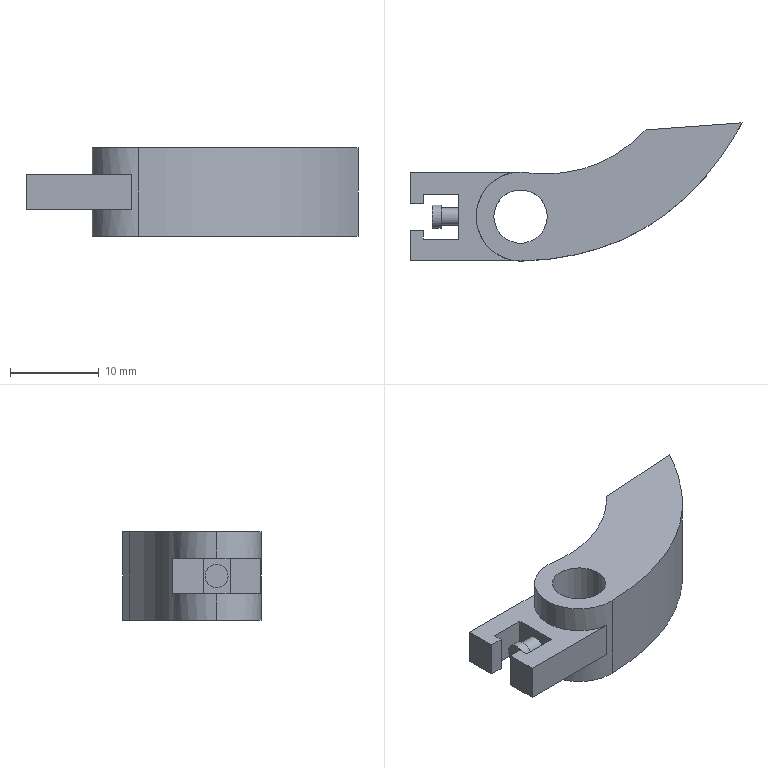Part | SolidWorks | features ICE 6, Extrusion 1 | 1 solid | 28 faces | box 37.304 x 15.525 x 10 mm | volume 2448 mm3 | plane 18 | cylinder 8 | spline 2 | commonest cylinder face diameters 2 x2 2.6 x2 6 x2 10 x2
STEP:
#1=CARTESIAN_POINT('',(-8.923,-1.3,5.));
#2=VERTEX_POINT('',#1);
#3=CARTESIAN_POINT('',(-8.923,1.3,5.));
#4=VERTEX_POINT('',#3);
#5=CARTESIAN_POINT('',(-8.923,0.,5.));
#6=DIRECTION('',(-1.,0.,0.));
#7=DIRECTION('',(0.,-1.,0.));
#8=AXIS2_PLACEMENT_3D('',#5,#6,#7);
#9=CIRCLE('',#8,1.3);
#10=EDGE_CURVE('',#2,#4,#9,.T.);
#11=ORIENTED_EDGE('',*,*,#10,.T.);
#12=CARTESIAN_POINT('',(-9.923,1.3,5.));
#13=VERTEX_POINT('',#12);
#14=CARTESIAN_POINT('',(-8.923,1.3,5.));
#15=DIRECTION('',(-1.,0.,0.));
#16=VECTOR('',#15,1000.);
#17=LINE('',#14,#16);
#18=EDGE_CURVE('',#4,#13,#17,.T.);
#19=ORIENTED_EDGE('',*,*,#18,.T.);
#20=CARTESIAN_POINT('',(-9.923,-1.3,5.));
#21=VERTEX_POINT('',#20);
#22=CARTESIAN_POINT('',(-9.923,0.,5.));
#23=DIRECTION('',(-1.,0.,0.));
#24=DIRECTION('',(0.,-1.,0.));
#25=AXIS2_PLACEMENT_3D('',#22,#23,#24);
#26=CIRCLE('',#25,1.3);
#27=EDGE_CURVE('',#21,#13,#26,.T.);
#28=ORIENTED_EDGE('',*,*,#27,.F.);
#29=CARTESIAN_POINT('',(-8.923,-1.3,5.));
#30=DIRECTION('',(-1.,0.,0.));
#31=VECTOR('',#30,1000.);
#32=LINE('',#29,#31);
#33=EDGE_CURVE('',#2,#21,#32,.T.);
#34=ORIENTED_EDGE('',*,*,#33,.F.);
#35=EDGE_LOOP('',(#11,#19,#28,#34));
#36=FACE_OUTER_BOUND('',#35,.T.);
#37=CARTESIAN_POINT('',(-8.923,0.,5.));
#38=DIRECTION('',(-1.,0.,0.));
#39=DIRECTION('',(0.,-1.,0.));
#40=AXIS2_PLACEMENT_3D('',#37,#38,#39);
#41=CYLINDRICAL_SURFACE('',#40,1.3);
#42=ADVANCED_FACE('',(#36),#41,.T.);
#43=CARTESIAN_POINT('',(-3.,0.,10.));
#44=VERTEX_POINT('',#43);
#45=CARTESIAN_POINT('',(3.,0.,10.));
#46=VERTEX_POINT('',#45);
#47=CARTESIAN_POINT('',(0.,0.,10.));
#48=DIRECTION('',(0.,0.,1.));
#49=DIRECTION('',(1.,0.,0.));
#50=AXIS2_PLACEMENT_3D('',#47,#48,#49);
#51=CIRCLE('',#50,3.);
#52=EDGE_CURVE('',#44,#46,#51,.T.);
#53=ORIENTED_EDGE('',*,*,#52,.T.);
#54=CARTESIAN_POINT('',(3.,0.,0.));
#55=VERTEX_POINT('',#54);
#56=CARTESIAN_POINT('',(3.,0.,10.));
#57=DIRECTION('',(0.,0.,-1.));
#58=VECTOR('',#57,1000.);
#59=LINE('',#56,#58);
#60=EDGE_CURVE('',#46,#55,#59,.T.);
#61=ORIENTED_EDGE('',*,*,#60,.T.);
#62=CARTESIAN_POINT('',(-3.,0.,0.));
#63=VERTEX_POINT('',#62);
#64=CARTESIAN_POINT('',(0.,0.,0.));
#65=DIRECTION('',(0.,0.,1.));
#66=DIRECTION('',(1.,0.,0.));
#67=AXIS2_PLACEMENT_3D('',#64,#65,#66);
#68=CIRCLE('',#67,3.);
#69=EDGE_CURVE('',#63,#55,#68,.T.);
#70=ORIENTED_EDGE('',*,*,#69,.F.);
#71=CARTESIAN_POINT('',(-3.,0.,10.));
#72=DIRECTION('',(0.,0.,-1.));
#73=VECTOR('',#72,1000.);
#74=LINE('',#71,#73);
#75=EDGE_CURVE('',#44,#63,#74,.T.);
#76=ORIENTED_EDGE('',*,*,#75,.F.);
#77=EDGE_LOOP('',(#53,#61,#70,#76));
#78=FACE_OUTER_BOUND('',#77,.T.);
#79=CARTESIAN_POINT('',(0.,0.,10.));
#80=DIRECTION('',(0.,0.,-1.));
#81=DIRECTION('',(-1.,0.,0.));
#82=AXIS2_PLACEMENT_3D('',#79,#80,#81);
#83=CYLINDRICAL_SURFACE('',#82,3.);
#84=ADVANCED_FACE('',(#78),#83,.F.);
#85=CARTESIAN_POINT('',(-5.,0.,10.));
#86=VERTEX_POINT('',#85);
#87=CARTESIAN_POINT('',(0.,-5.,10.));
#88=VERTEX_POINT('',#87);
#89=CARTESIAN_POINT('',(0.,0.,10.));
#90=DIRECTION('',(0.,0.,1.));
#91=DIRECTION('',(1.,0.,0.));
#92=AXIS2_PLACEMENT_3D('',#89,#90,#91);
#93=CIRCLE('',#92,5.);
#94=EDGE_CURVE('',#86,#88,#93,.T.);
#95=ORIENTED_EDGE('',*,*,#94,.F.);
#96=CARTESIAN_POINT('',(-5.,0.,7.));
#97=VERTEX_POINT('',#96);
#98=CARTESIAN_POINT('',(-5.,0.,10.));
#99=DIRECTION('',(0.,0.,-1.));
#100=VECTOR('',#99,1000.);
#101=LINE('',#98,#100);
#102=EDGE_CURVE('',#86,#97,#101,.T.);
#103=ORIENTED_EDGE('',*,*,#102,.T.);
#104=CARTESIAN_POINT('',(-0.589,-4.965,7.));
#105=VERTEX_POINT('',#104);
#106=CARTESIAN_POINT('',(0.,0.,7.));
#107=DIRECTION('',(0.,0.,1.));
#108=DIRECTION('',(1.,0.,0.));
#109=AXIS2_PLACEMENT_3D('',#106,#107,#108);
#110=CIRCLE('',#109,5.);
#111=EDGE_CURVE('',#97,#105,#110,.T.);
#112=ORIENTED_EDGE('',*,*,#111,.T.);
#113=CARTESIAN_POINT('',(-0.589,-4.965,3.));
#114=VERTEX_POINT('',#113);
#115=CARTESIAN_POINT('',(-0.589,-4.965,10.));
#116=DIRECTION('',(0.,0.,-1.));
#117=VECTOR('',#116,1000.);
#118=LINE('',#115,#117);
#119=EDGE_CURVE('',#105,#114,#118,.T.);
#120=ORIENTED_EDGE('',*,*,#119,.T.);
#121=CARTESIAN_POINT('',(-5.,0.,3.));
#122=VERTEX_POINT('',#121);
#123=CARTESIAN_POINT('',(0.,0.,3.));
#124=DIRECTION('',(0.,0.,1.));
#125=DIRECTION('',(1.,0.,0.));
#126=AXIS2_PLACEMENT_3D('',#123,#124,#125);
#127=CIRCLE('',#126,5.);
#128=EDGE_CURVE('',#122,#114,#127,.T.);
#129=ORIENTED_EDGE('',*,*,#128,.F.);
#130=CARTESIAN_POINT('',(-5.,0.,0.));
#131=VERTEX_POINT('',#130);
#132=CARTESIAN_POINT('',(-5.,0.,10.));
#133=DIRECTION('',(0.,0.,-1.));
#134=VECTOR('',#133,1000.);
#135=LINE('',#132,#134);
#136=EDGE_CURVE('',#122,#131,#135,.T.);
#137=ORIENTED_EDGE('',*,*,#136,.T.);
#138=CARTESIAN_POINT('',(0.,-5.,0.));
#139=VERTEX_POINT('',#138);
#140=CARTESIAN_POINT('',(0.,0.,0.));
#141=DIRECTION('',(0.,0.,1.));
#142=DIRECTION('',(1.,0.,0.));
#143=AXIS2_PLACEMENT_3D('',#140,#141,#142);
#144=CIRCLE('',#143,5.);
#145=EDGE_CURVE('',#131,#139,#144,.T.);
#146=ORIENTED_EDGE('',*,*,#145,.T.);
#147=CARTESIAN_POINT('',(0.2548,-4.994,0.));
#148=VERTEX_POINT('',#147);
#149=CARTESIAN_POINT('',(0.,-5.,0.));
#150=CARTESIAN_POINT('',(0.08497,-5.,0.));
#151=CARTESIAN_POINT('',(0.1699,-4.998,0.));
#152=CARTESIAN_POINT('',(0.2548,-4.994,0.));
#153=B_SPLINE_CURVE_WITH_KNOTS('',3,(#149,#150,#151,#152),.UNSPECIFIED.,.F.,.F.,(4,4),(0.,1.),.UNSPECIFIED.);
#154=EDGE_CURVE('',#139,#148,#153,.T.);
#155=ORIENTED_EDGE('',*,*,#154,.T.);
#156=CARTESIAN_POINT('',(0.2548,-4.994,10.));
#157=VERTEX_POINT('',#156);
#158=CARTESIAN_POINT('',(0.2548,-4.994,0.));
#159=DIRECTION('',(0.,0.,1.));
#160=VECTOR('',#159,1000.);
#161=LINE('',#158,#160);
#162=EDGE_CURVE('',#148,#157,#161,.T.);
#163=ORIENTED_EDGE('',*,*,#162,.T.);
#164=CARTESIAN_POINT('',(0.,-5.,10.));
#165=CARTESIAN_POINT('',(0.08493,-4.998,10.));
#166=CARTESIAN_POINT('',(0.1699,-4.996,10.));
#167=CARTESIAN_POINT('',(0.2548,-4.994,10.));
#168=B_SPLINE_CURVE_WITH_KNOTS('',3,(#164,#165,#166,#167),.UNSPECIFIED.,.F.,.F.,(4,4),(0.,1.),.UNSPECIFIED.);
#169=EDGE_CURVE('',#88,#157,#168,.T.);
#170=ORIENTED_EDGE('',*,*,#169,.F.);
#171=EDGE_LOOP('',(#95,#103,#112,#120,#129,#137,#146,#155,#163,#170));
#172=FACE_OUTER_BOUND('',#171,.T.);
#173=CARTESIAN_POINT('',(0.,0.,10.));
#174=DIRECTION('',(0.,0.,-1.));
#175=DIRECTION('',(-1.,0.,0.));
#176=AXIS2_PLACEMENT_3D('',#173,#174,#175);
#177=CYLINDRICAL_SURFACE('',#176,5.);
#178=ADVANCED_FACE('',(#172),#177,.T.);
#179=CARTESIAN_POINT('',(-8.923,-1.,5.));
#180=VERTEX_POINT('',#179);
#181=CARTESIAN_POINT('',(-8.923,1.,5.));
#182=VERTEX_POINT('',#181);
#183=CARTESIAN_POINT('',(-8.923,0.,5.));
#184=DIRECTION('',(-1.,0.,0.));
#185=DIRECTION('',(0.,-1.,0.));
#186=AXIS2_PLACEMENT_3D('',#183,#184,#185);
#187=CIRCLE('',#186,1.);
#188=EDGE_CURVE('',#180,#182,#187,.T.);
#189=ORIENTED_EDGE('',*,*,#188,.F.);
#190=CARTESIAN_POINT('',(-6.923,-1.,5.));
#191=VERTEX_POINT('',#190);
#192=CARTESIAN_POINT('',(-9.923,-1.,5.));
#193=DIRECTION('',(1.,0.,0.));
#194=VECTOR('',#193,1000.);
#195=LINE('',#192,#194);
#196=EDGE_CURVE('',#180,#191,#195,.T.);
#197=ORIENTED_EDGE('',*,*,#196,.T.);
#198=CARTESIAN_POINT('',(-6.923,1.,5.));
#199=VERTEX_POINT('',#198);
#200=CARTESIAN_POINT('',(-6.923,0.,5.));
#201=DIRECTION('',(-1.,0.,0.));
#202=DIRECTION('',(0.,1.,0.));
#203=AXIS2_PLACEMENT_3D('',#200,#201,#202);
#204=CIRCLE('',#203,1.);
#205=EDGE_CURVE('',#191,#199,#204,.T.);
#206=ORIENTED_EDGE('',*,*,#205,.T.);
#207=CARTESIAN_POINT('',(-9.923,1.,5.));
#208=DIRECTION('',(1.,0.,0.));
#209=VECTOR('',#208,1000.);
#210=LINE('',#207,#209);
#211=EDGE_CURVE('',#182,#199,#210,.T.);
#212=ORIENTED_EDGE('',*,*,#211,.F.);
#213=EDGE_LOOP('',(#189,#197,#206,#212));
#214=FACE_OUTER_BOUND('',#213,.T.);
#215=CARTESIAN_POINT('',(-9.923,0.,5.));
#216=DIRECTION('',(1.,0.,0.));
#217=DIRECTION('',(0.,1.,0.));
#218=AXIS2_PLACEMENT_3D('',#215,#216,#217);
#219=CYLINDRICAL_SURFACE('',#218,1.);
#220=ADVANCED_FACE('',(#214),#219,.T.);
#221=ORIENTED_EDGE('',*,*,#196,.F.);
#222=CARTESIAN_POINT('',(-8.923,0.,5.));
#223=DIRECTION('',(-1.,0.,0.));
#224=DIRECTION('',(0.,-1.,0.));
#225=AXIS2_PLACEMENT_3D('',#222,#223,#224);
#226=CIRCLE('',#225,1.);
#227=EDGE_CURVE('',#182,#180,#226,.T.);
#228=ORIENTED_EDGE('',*,*,#227,.F.);
#229=ORIENTED_EDGE('',*,*,#211,.T.);
#230=CARTESIAN_POINT('',(-6.923,0.,5.));
#231=DIRECTION('',(-1.,0.,0.));
#232=DIRECTION('',(0.,1.,0.));
#233=AXIS2_PLACEMENT_3D('',#230,#231,#232);
#234=CIRCLE('',#233,1.);
#235=EDGE_CURVE('',#199,#191,#234,.T.);
#236=ORIENTED_EDGE('',*,*,#235,.T.);
#237=EDGE_LOOP('',(#221,#228,#229,#236));
#238=FACE_OUTER_BOUND('',#237,.T.);
#239=CARTESIAN_POINT('',(-9.923,0.,5.));
#240=DIRECTION('',(1.,0.,0.));
#241=DIRECTION('',(0.,1.,0.));
#242=AXIS2_PLACEMENT_3D('',#239,#240,#241);
#243=CYLINDRICAL_SURFACE('',#242,1.);
#244=ADVANCED_FACE('',(#238),#243,.T.);
#245=CARTESIAN_POINT('',(-12.423,1.465,7.));
#246=VERTEX_POINT('',#245);
#247=CARTESIAN_POINT('',(-12.423,1.465,3.));
#248=VERTEX_POINT('',#247);
#249=CARTESIAN_POINT('',(-12.423,1.465,0.));
#250=DIRECTION('',(0.,0.,-1.));
#251=VECTOR('',#250,1000.);
#252=LINE('',#249,#251);
#253=EDGE_CURVE('',#246,#248,#252,.T.);
#254=ORIENTED_EDGE('',*,*,#253,.F.);
#255=CARTESIAN_POINT('',(-12.423,4.965,7.));
#256=VERTEX_POINT('',#255);
#257=CARTESIAN_POINT('',(-12.423,4.965,7.));
#258=DIRECTION('',(0.,1.,0.));
#259=VECTOR('',#258,1000.);
#260=LINE('',#257,#259);
#261=EDGE_CURVE('',#246,#256,#260,.T.);
#262=ORIENTED_EDGE('',*,*,#261,.T.);
#263=CARTESIAN_POINT('',(-12.423,4.965,3.));
#264=VERTEX_POINT('',#263);
#265=CARTESIAN_POINT('',(-12.423,4.965,3.));
#266=DIRECTION('',(0.,0.,-1.));
#267=VECTOR('',#266,1000.);
#268=LINE('',#265,#267);
#269=EDGE_CURVE('',#256,#264,#268,.T.);
#270=ORIENTED_EDGE('',*,*,#269,.T.);
#271=CARTESIAN_POINT('',(-12.423,4.965,3.));
#272=DIRECTION('',(0.,-1.,0.));
#273=VECTOR('',#272,1000.);
#274=LINE('',#271,#273);
#275=EDGE_CURVE('',#264,#248,#274,.T.);
#276=ORIENTED_EDGE('',*,*,#275,.T.);
#277=EDGE_LOOP('',(#254,#262,#270,#276));
#278=FACE_OUTER_BOUND('',#277,.T.);
#279=CARTESIAN_POINT('',(-12.423,0.,0.));
#280=DIRECTION('',(-1.,0.,0.));
#281=DIRECTION('',(0.,0.,1.));
#282=AXIS2_PLACEMENT_3D('',#279,#280,#281);
#283=PLANE('',#282);
#284=ADVANCED_FACE('',(#278),#283,.T.);
#285=CARTESIAN_POINT('',(-12.423,-4.965,7.));
#286=VERTEX_POINT('',#285);
#287=CARTESIAN_POINT('',(-20.423,-4.965,7.));
#288=DIRECTION('',(1.,0.,0.));
#289=VECTOR('',#288,1000.);
#290=LINE('',#287,#289);
#291=EDGE_CURVE('',#286,#105,#290,.T.);
#292=ORIENTED_EDGE('',*,*,#291,.F.);
#293=CARTESIAN_POINT('',(-12.423,-4.965,3.));
#294=VERTEX_POINT('',#293);
#295=CARTESIAN_POINT('',(-12.423,-4.965,3.));
#296=DIRECTION('',(0.,0.,1.));
#297=VECTOR('',#296,1000.);
#298=LINE('',#295,#297);
#299=EDGE_CURVE('',#294,#286,#298,.T.);
#300=ORIENTED_EDGE('',*,*,#299,.F.);
#301=CARTESIAN_POINT('',(-20.423,-4.965,3.));
#302=DIRECTION('',(1.,0.,0.));
#303=VECTOR('',#302,1000.);
#304=LINE('',#301,#303);
#305=EDGE_CURVE('',#294,#114,#304,.T.);
#306=ORIENTED_EDGE('',*,*,#305,.T.);
#307=ORIENTED_EDGE('',*,*,#119,.F.);
#308=EDGE_LOOP('',(#292,#300,#306,#307));
#309=FACE_OUTER_BOUND('',#308,.T.);
#310=CARTESIAN_POINT('',(-20.423,-4.965,3.));
#311=DIRECTION('',(0.,-1.,0.));
#312=DIRECTION('',(0.,0.,-1.));
#313=AXIS2_PLACEMENT_3D('',#310,#311,#312);
#314=PLANE('',#313);
#315=ADVANCED_FACE('',(#309),#314,.T.);
#316=CARTESIAN_POINT('',(-0.589,4.965,3.));
#317=VERTEX_POINT('',#316);
#318=CARTESIAN_POINT('',(-20.423,4.965,3.));
#319=DIRECTION('',(-1.,0.,0.));
#320=VECTOR('',#319,1000.);
#321=LINE('',#318,#320);
#322=EDGE_CURVE('',#317,#264,#321,.T.);
#323=ORIENTED_EDGE('',*,*,#322,.T.);
#324=ORIENTED_EDGE('',*,*,#269,.F.);
#325=CARTESIAN_POINT('',(-0.589,4.965,7.));
#326=VERTEX_POINT('',#325);
#327=CARTESIAN_POINT('',(-20.423,4.965,7.));
#328=DIRECTION('',(-1.,0.,0.));
#329=VECTOR('',#328,1000.);
#330=LINE('',#327,#329);
#331=EDGE_CURVE('',#326,#256,#330,.T.);
#332=ORIENTED_EDGE('',*,*,#331,.F.);
#333=CARTESIAN_POINT('',(-0.589,4.965,10.));
#334=DIRECTION('',(0.,0.,1.));
#335=VECTOR('',#334,1000.);
#336=LINE('',#333,#335);
#337=EDGE_CURVE('',#317,#326,#336,.T.);
#338=ORIENTED_EDGE('',*,*,#337,.F.);
#339=EDGE_LOOP('',(#323,#324,#332,#338));
#340=FACE_OUTER_BOUND('',#339,.T.);
#341=CARTESIAN_POINT('',(-20.423,4.965,3.));
#342=DIRECTION('',(0.,1.,0.));
#343=DIRECTION('',(0.,0.,1.));
#344=AXIS2_PLACEMENT_3D('',#341,#342,#343);
#345=PLANE('',#344);
#346=ADVANCED_FACE('',(#340),#345,.T.);
#347=CARTESIAN_POINT('',(-10.923,2.465,3.));
#348=VERTEX_POINT('',#347);
#349=CARTESIAN_POINT('',(-10.923,1.465,3.));
#350=VERTEX_POINT('',#349);
#351=CARTESIAN_POINT('',(-10.923,0.,3.));
#352=DIRECTION('',(0.,-1.,0.));
#353=VECTOR('',#352,1000.);
#354=LINE('',#351,#353);
#355=EDGE_CURVE('',#348,#350,#354,.T.);
#356=ORIENTED_EDGE('',*,*,#355,.T.);
#357=CARTESIAN_POINT('',(0.,1.465,3.));
#358=DIRECTION('',(-1.,0.,0.));
#359=VECTOR('',#358,1000.);
#360=LINE('',#357,#359);
#361=EDGE_CURVE('',#350,#248,#360,.T.);
#362=ORIENTED_EDGE('',*,*,#361,.T.);
#363=ORIENTED_EDGE('',*,*,#275,.F.);
#364=ORIENTED_EDGE('',*,*,#322,.F.);
#365=CARTESIAN_POINT('',(0.,0.,3.));
#366=DIRECTION('',(0.,0.,1.));
#367=DIRECTION('',(1.,0.,0.));
#368=AXIS2_PLACEMENT_3D('',#365,#366,#367);
#369=CIRCLE('',#368,5.);
#370=EDGE_CURVE('',#317,#122,#369,.T.);
#371=ORIENTED_EDGE('',*,*,#370,.T.);
#372=ORIENTED_EDGE('',*,*,#128,.T.);
#373=ORIENTED_EDGE('',*,*,#305,.F.);
#374=CARTESIAN_POINT('',(-12.423,-1.535,3.));
#375=VERTEX_POINT('',#374);
#376=CARTESIAN_POINT('',(-12.423,4.965,3.));
#377=DIRECTION('',(0.,-1.,0.));
#378=VECTOR('',#377,1000.);
#379=LINE('',#376,#378);
#380=EDGE_CURVE('',#375,#294,#379,.T.);
#381=ORIENTED_EDGE('',*,*,#380,.F.);
#382=CARTESIAN_POINT('',(-10.923,-1.535,3.));
#383=VERTEX_POINT('',#382);
#384=CARTESIAN_POINT('',(0.,-1.535,3.));
#385=DIRECTION('',(1.,0.,0.));
#386=VECTOR('',#385,1000.);
#387=LINE('',#384,#386);
#388=EDGE_CURVE('',#375,#383,#387,.T.);
#389=ORIENTED_EDGE('',*,*,#388,.T.);
#390=CARTESIAN_POINT('',(-10.923,-2.535,3.));
#391=VERTEX_POINT('',#390);
#392=CARTESIAN_POINT('',(-10.923,0.,3.));
#393=DIRECTION('',(0.,-1.,0.));
#394=VECTOR('',#393,1000.);
#395=LINE('',#392,#394);
#396=EDGE_CURVE('',#383,#391,#395,.T.);
#397=ORIENTED_EDGE('',*,*,#396,.T.);
#398=CARTESIAN_POINT('',(-6.923,-2.535,3.));
#399=VERTEX_POINT('',#398);
#400=CARTESIAN_POINT('',(0.,-2.535,3.));
#401=DIRECTION('',(1.,0.,0.));
#402=VECTOR('',#401,1000.);
#403=LINE('',#400,#402);
#404=EDGE_CURVE('',#391,#399,#403,.T.);
#405=ORIENTED_EDGE('',*,*,#404,.T.);
#406=CARTESIAN_POINT('',(-6.923,2.465,3.));
#407=VERTEX_POINT('',#406);
#408=CARTESIAN_POINT('',(-6.923,0.,3.));
#409=DIRECTION('',(0.,1.,0.));
#410=VECTOR('',#409,1000.);
#411=LINE('',#408,#410);
#412=EDGE_CURVE('',#399,#407,#411,.T.);
#413=ORIENTED_EDGE('',*,*,#412,.T.);
#414=CARTESIAN_POINT('',(0.,2.465,3.));
#415=DIRECTION('',(-1.,0.,0.));
#416=VECTOR('',#415,1000.);
#417=LINE('',#414,#416);
#418=EDGE_CURVE('',#407,#348,#417,.T.);
#419=ORIENTED_EDGE('',*,*,#418,.T.);
#420=EDGE_LOOP('',(#356,#362,#363,#364,#371,#372,#373,#381,#389,#397,#405,#413,#419));
#421=FACE_OUTER_BOUND('',#420,.T.);
#422=CARTESIAN_POINT('',(0.,0.,3.));
#423=DIRECTION('',(0.,0.,1.));
#424=DIRECTION('',(1.,0.,0.));
#425=AXIS2_PLACEMENT_3D('',#422,#423,#424);
#426=PLANE('',#425);
#427=ADVANCED_FACE('',(#421),#426,.F.);
#428=CARTESIAN_POINT('',(-10.923,1.465,7.));
#429=VERTEX_POINT('',#428);
#430=CARTESIAN_POINT('',(-12.423,1.465,7.));
#431=DIRECTION('',(-1.,0.,0.));
#432=VECTOR('',#431,1000.);
#433=LINE('',#430,#432);
#434=EDGE_CURVE('',#429,#246,#433,.T.);
#435=ORIENTED_EDGE('',*,*,#434,.F.);
#436=CARTESIAN_POINT('',(-10.923,2.465,7.));
#437=VERTEX_POINT('',#436);
#438=CARTESIAN_POINT('',(-10.923,1.465,7.));
#439=DIRECTION('',(0.,-1.,0.));
#440=VECTOR('',#439,1000.);
#441=LINE('',#438,#440);
#442=EDGE_CURVE('',#437,#429,#441,.T.);
#443=ORIENTED_EDGE('',*,*,#442,.F.);
#444=CARTESIAN_POINT('',(-6.923,2.465,7.));
#445=VERTEX_POINT('',#444);
#446=CARTESIAN_POINT('',(-10.923,2.465,7.));
#447=DIRECTION('',(-1.,0.,0.));
#448=VECTOR('',#447,1000.);
#449=LINE('',#446,#448);
#450=EDGE_CURVE('',#445,#437,#449,.T.);
#451=ORIENTED_EDGE('',*,*,#450,.F.);
#452=CARTESIAN_POINT('',(-6.923,-2.535,7.));
#453=VERTEX_POINT('',#452);
#454=CARTESIAN_POINT('',(-6.923,2.465,7.));
#455=DIRECTION('',(0.,1.,0.));
#456=VECTOR('',#455,1000.);
#457=LINE('',#454,#456);
#458=EDGE_CURVE('',#453,#445,#457,.T.);
#459=ORIENTED_EDGE('',*,*,#458,.F.);
#460=CARTESIAN_POINT('',(-10.923,-2.535,7.));
#461=VERTEX_POINT('',#460);
#462=CARTESIAN_POINT('',(-6.923,-2.535,7.));
#463=DIRECTION('',(1.,0.,0.));
#464=VECTOR('',#463,1000.);
#465=LINE('',#462,#464);
#466=EDGE_CURVE('',#461,#453,#465,.T.);
#467=ORIENTED_EDGE('',*,*,#466,.F.);
#468=CARTESIAN_POINT('',(-10.923,-1.535,7.));
#469=VERTEX_POINT('',#468);
#470=CARTESIAN_POINT('',(-10.923,-2.535,7.));
#471=DIRECTION('',(0.,-1.,0.));
#472=VECTOR('',#471,1000.);
#473=LINE('',#470,#472);
#474=EDGE_CURVE('',#469,#461,#473,.T.);
#475=ORIENTED_EDGE('',*,*,#474,.F.);
#476=CARTESIAN_POINT('',(-12.423,-1.535,7.));
#477=VERTEX_POINT('',#476);
#478=CARTESIAN_POINT('',(-10.923,-1.535,7.));
#479=DIRECTION('',(1.,0.,0.));
#480=VECTOR('',#479,1000.);
#481=LINE('',#478,#480);
#482=EDGE_CURVE('',#477,#469,#481,.T.);
#483=ORIENTED_EDGE('',*,*,#482,.F.);
#484=CARTESIAN_POINT('',(-12.423,4.965,7.));
#485=DIRECTION('',(0.,1.,0.));
#486=VECTOR('',#485,1000.);
#487=LINE('',#484,#486);
#488=EDGE_CURVE('',#286,#477,#487,.T.);
#489=ORIENTED_EDGE('',*,*,#488,.F.);
#490=ORIENTED_EDGE('',*,*,#291,.T.);
#491=ORIENTED_EDGE('',*,*,#111,.F.);
#492=CARTESIAN_POINT('',(0.,0.,7.));
#493=DIRECTION('',(0.,0.,1.));
#494=DIRECTION('',(1.,0.,0.));
#495=AXIS2_PLACEMENT_3D('',#492,#493,#494);
#496=CIRCLE('',#495,5.);
#497=EDGE_CURVE('',#326,#97,#496,.T.);
#498=ORIENTED_EDGE('',*,*,#497,.F.);
#499=ORIENTED_EDGE('',*,*,#331,.T.);
#500=ORIENTED_EDGE('',*,*,#261,.F.);
#501=EDGE_LOOP('',(#435,#443,#451,#459,#467,#475,#483,#489,#490,#491,#498,#499,#500));
#502=FACE_OUTER_BOUND('',#501,.T.);
#503=CARTESIAN_POINT('',(0.,0.,7.));
#504=DIRECTION('',(0.,0.,1.));
#505=DIRECTION('',(1.,0.,0.));
#506=AXIS2_PLACEMENT_3D('',#503,#504,#505);
#507=PLANE('',#506);
#508=ADVANCED_FACE('',(#502),#507,.T.);
#509=ORIENTED_EDGE('',*,*,#102,.F.);
#510=CARTESIAN_POINT('',(1.168,4.862,10.));
#511=VERTEX_POINT('',#510);
#512=CARTESIAN_POINT('',(0.,0.,10.));
#513=DIRECTION('',(0.,0.,1.));
#514=DIRECTION('',(1.,0.,0.));
#515=AXIS2_PLACEMENT_3D('',#512,#513,#514);
#516=CIRCLE('',#515,5.);
#517=EDGE_CURVE('',#511,#86,#516,.T.);
#518=ORIENTED_EDGE('',*,*,#517,.F.);
#519=CARTESIAN_POINT('',(1.168,4.862,0.));
#520=VERTEX_POINT('',#519);
#521=CARTESIAN_POINT('',(1.168,4.862,0.));
#522=DIRECTION('',(0.,0.,-1.));
#523=VECTOR('',#522,1000.);
#524=LINE('',#521,#523);
#525=EDGE_CURVE('',#511,#520,#524,.T.);
#526=ORIENTED_EDGE('',*,*,#525,.T.);
#527=CARTESIAN_POINT('',(0.,0.,0.));
#528=DIRECTION('',(0.,0.,1.));
#529=DIRECTION('',(1.,0.,0.));
#530=AXIS2_PLACEMENT_3D('',#527,#528,#529);
#531=CIRCLE('',#530,5.);
#532=EDGE_CURVE('',#520,#131,#531,.T.);
#533=ORIENTED_EDGE('',*,*,#532,.T.);
#534=ORIENTED_EDGE('',*,*,#136,.F.);
#535=ORIENTED_EDGE('',*,*,#370,.F.);
#536=ORIENTED_EDGE('',*,*,#337,.T.);
#537=ORIENTED_EDGE('',*,*,#497,.T.);
#538=EDGE_LOOP('',(#509,#518,#526,#533,#534,#535,#536,#537));
#539=FACE_OUTER_BOUND('',#538,.T.);
#540=CARTESIAN_POINT('',(0.,0.,10.));
#541=DIRECTION('',(0.,0.,-1.));
#542=DIRECTION('',(-1.,0.,0.));
#543=AXIS2_PLACEMENT_3D('',#540,#541,#542);
#544=CYLINDRICAL_SURFACE('',#543,5.);
#545=ADVANCED_FACE('',(#539),#544,.T.);
#546=ORIENTED_EDGE('',*,*,#517,.T.);
#547=ORIENTED_EDGE('',*,*,#94,.T.);
#548=ORIENTED_EDGE('',*,*,#169,.T.);
#549=CARTESIAN_POINT('',(24.88,10.525,10.));
#550=VERTEX_POINT('',#549);
#551=CARTESIAN_POINT('',(0.2548,-4.994,10.));
#552=CARTESIAN_POINT('',(16.753,-4.516,10.));
#553=CARTESIAN_POINT('',(24.88,10.525,10.));
#554=B_SPLINE_CURVE_WITH_KNOTS('',2,(#551,#552,#553),.UNSPECIFIED.,.F.,.F.,(3,3),(0.007648,1.),.UNSPECIFIED.);
#555=EDGE_CURVE('',#157,#550,#554,.T.);
#556=ORIENTED_EDGE('',*,*,#555,.T.);
#557=CARTESIAN_POINT('',(14.105,9.738,10.));
#558=VERTEX_POINT('',#557);
#559=CARTESIAN_POINT('',(24.88,10.525,10.));
#560=DIRECTION('',(-0.9973,-0.07288,0.));
#561=VECTOR('',#560,1000.);
#562=LINE('',#559,#561);
#563=EDGE_CURVE('',#550,#558,#562,.T.);
#564=ORIENTED_EDGE('',*,*,#563,.T.);
#565=CARTESIAN_POINT('',(14.105,9.738,10.));
#566=CARTESIAN_POINT('',(8.733,4.193,10.));
#567=CARTESIAN_POINT('',(1.168,4.862,10.));
#568=B_SPLINE_CURVE_WITH_KNOTS('',2,(#565,#566,#567),.UNSPECIFIED.,.F.,.F.,(3,3),(0.,0.9291),.UNSPECIFIED.);
#569=EDGE_CURVE('',#558,#511,#568,.T.);
#570=ORIENTED_EDGE('',*,*,#569,.T.);
#571=EDGE_LOOP('',(#546,#547,#548,#556,#564,#570));
#572=FACE_OUTER_BOUND('',#571,.T.);
#573=ORIENTED_EDGE('',*,*,#52,.F.);
#574=CARTESIAN_POINT('',(0.,0.,10.));
#575=DIRECTION('',(0.,0.,1.));
#576=DIRECTION('',(1.,0.,0.));
#577=AXIS2_PLACEMENT_3D('',#574,#575,#576);
#578=CIRCLE('',#577,3.);
#579=EDGE_CURVE('',#46,#44,#578,.T.);
#580=ORIENTED_EDGE('',*,*,#579,.F.);
#581=EDGE_LOOP('',(#573,#580));
#582=FACE_BOUND('',#581,.T.);
#583=CARTESIAN_POINT('',(0.,0.,10.));
#584=DIRECTION('',(0.,0.,1.));
#585=DIRECTION('',(1.,0.,0.));
#586=AXIS2_PLACEMENT_3D('',#583,#584,#585);
#587=PLANE('',#586);
#588=ADVANCED_FACE('',(#572,#582),#587,.T.);
#589=ORIENTED_EDGE('',*,*,#532,.F.);
#590=CARTESIAN_POINT('',(14.105,9.738,0.));
#591=VERTEX_POINT('',#590);
#592=CARTESIAN_POINT('',(14.105,9.738,0.));
#593=CARTESIAN_POINT('',(8.733,4.193,0.));
#594=CARTESIAN_POINT('',(1.168,4.862,0.));
#595=B_SPLINE_CURVE_WITH_KNOTS('',2,(#592,#593,#594),.UNSPECIFIED.,.F.,.F.,(3,3),(0.,0.9291),.UNSPECIFIED.);
#596=EDGE_CURVE('',#591,#520,#595,.T.);
#597=ORIENTED_EDGE('',*,*,#596,.F.);
#598=CARTESIAN_POINT('',(24.88,10.525,0.));
#599=VERTEX_POINT('',#598);
#600=CARTESIAN_POINT('',(24.88,10.525,0.));
#601=DIRECTION('',(-0.9973,-0.07288,0.));
#602=VECTOR('',#601,1000.);
#603=LINE('',#600,#602);
#604=EDGE_CURVE('',#599,#591,#603,.T.);
#605=ORIENTED_EDGE('',*,*,#604,.F.);
#606=CARTESIAN_POINT('',(0.2548,-4.994,0.));
#607=CARTESIAN_POINT('',(16.753,-4.516,0.));
#608=CARTESIAN_POINT('',(24.88,10.525,0.));
#609=B_SPLINE_CURVE_WITH_KNOTS('',2,(#606,#607,#608),.UNSPECIFIED.,.F.,.F.,(3,3),(0.007648,1.),.UNSPECIFIED.);
#610=EDGE_CURVE('',#148,#599,#609,.T.);
#611=ORIENTED_EDGE('',*,*,#610,.F.);
#612=ORIENTED_EDGE('',*,*,#154,.F.);
#613=ORIENTED_EDGE('',*,*,#145,.F.);
#614=EDGE_LOOP('',(#589,#597,#605,#611,#612,#613));
#615=FACE_OUTER_BOUND('',#614,.T.);
#616=ORIENTED_EDGE('',*,*,#69,.T.);
#617=CARTESIAN_POINT('',(0.,0.,0.));
#618=DIRECTION('',(0.,0.,1.));
#619=DIRECTION('',(1.,0.,0.));
#620=AXIS2_PLACEMENT_3D('',#617,#618,#619);
#621=CIRCLE('',#620,3.);
#622=EDGE_CURVE('',#55,#63,#621,.T.);
#623=ORIENTED_EDGE('',*,*,#622,.T.);
#624=EDGE_LOOP('',(#616,#623));
#625=FACE_BOUND('',#624,.T.);
#626=CARTESIAN_POINT('',(0.,0.,0.));
#627=DIRECTION('',(0.,0.,1.));
#628=DIRECTION('',(1.,0.,0.));
#629=AXIS2_PLACEMENT_3D('',#626,#627,#628);
#630=PLANE('',#629);
#631=ADVANCED_FACE('',(#615,#625),#630,.F.);
#632=ORIENTED_EDGE('',*,*,#60,.F.);
#633=ORIENTED_EDGE('',*,*,#579,.T.);
#634=ORIENTED_EDGE('',*,*,#75,.T.);
#635=ORIENTED_EDGE('',*,*,#622,.F.);
#636=EDGE_LOOP('',(#632,#633,#634,#635));
#637=FACE_OUTER_BOUND('',#636,.T.);
#638=CARTESIAN_POINT('',(0.,0.,10.));
#639=DIRECTION('',(0.,0.,-1.));
#640=DIRECTION('',(-1.,0.,0.));
#641=AXIS2_PLACEMENT_3D('',#638,#639,#640);
#642=CYLINDRICAL_SURFACE('',#641,3.);
#643=ADVANCED_FACE('',(#637),#642,.F.);
#644=ORIENTED_EDGE('',*,*,#162,.F.);
#645=ORIENTED_EDGE('',*,*,#610,.T.);
#646=CARTESIAN_POINT('',(24.88,10.525,0.));
#647=DIRECTION('',(0.,0.,1.));
#648=VECTOR('',#647,1000.);
#649=LINE('',#646,#648);
#650=EDGE_CURVE('',#599,#550,#649,.T.);
#651=ORIENTED_EDGE('',*,*,#650,.T.);
#652=ORIENTED_EDGE('',*,*,#555,.F.);
#653=EDGE_LOOP('',(#644,#645,#651,#652));
#654=FACE_OUTER_BOUND('',#653,.T.);
#655=CARTESIAN_POINT('',(0.2548,-4.994,0.));
#656=CARTESIAN_POINT('',(0.2548,-4.994,10.));
#657=CARTESIAN_POINT('',(16.753,-4.516,0.));
#658=CARTESIAN_POINT('',(16.753,-4.516,10.));
#659=CARTESIAN_POINT('',(24.88,10.525,0.));
#660=CARTESIAN_POINT('',(24.88,10.525,10.));
#661=B_SPLINE_SURFACE_WITH_KNOTS('',2,1,((#655,#656),(#657,#658),(#659,#660)),.UNSPECIFIED.,.F.,.F.,.F.,(3,3),(2,2),(0.007648,1.),(0.,1.),.UNSPECIFIED.);
#662=ADVANCED_FACE('',(#654),#661,.T.);
#663=ORIENTED_EDGE('',*,*,#525,.F.);
#664=ORIENTED_EDGE('',*,*,#569,.F.);
#665=CARTESIAN_POINT('',(14.105,9.738,0.));
#666=DIRECTION('',(0.,0.,1.));
#667=VECTOR('',#666,1000.);
#668=LINE('',#665,#667);
#669=EDGE_CURVE('',#591,#558,#668,.T.);
#670=ORIENTED_EDGE('',*,*,#669,.F.);
#671=ORIENTED_EDGE('',*,*,#596,.T.);
#672=EDGE_LOOP('',(#663,#664,#670,#671));
#673=FACE_OUTER_BOUND('',#672,.T.);
#674=CARTESIAN_POINT('',(14.105,9.738,0.));
#675=CARTESIAN_POINT('',(14.105,9.738,10.));
#676=CARTESIAN_POINT('',(8.733,4.193,0.));
#677=CARTESIAN_POINT('',(8.733,4.193,10.));
#678=CARTESIAN_POINT('',(1.168,4.862,0.));
#679=CARTESIAN_POINT('',(1.168,4.862,10.));
#680=B_SPLINE_SURFACE_WITH_KNOTS('',2,1,((#674,#675),(#676,#677),(#678,#679)),.UNSPECIFIED.,.F.,.F.,.F.,(3,3),(2,2),(0.,0.9291),(0.,1.),.UNSPECIFIED.);
#681=ADVANCED_FACE('',(#673),#680,.T.);
#682=ORIENTED_EDGE('',*,*,#563,.F.);
#683=ORIENTED_EDGE('',*,*,#650,.F.);
#684=ORIENTED_EDGE('',*,*,#604,.T.);
#685=ORIENTED_EDGE('',*,*,#669,.T.);
#686=EDGE_LOOP('',(#682,#683,#684,#685));
#687=FACE_OUTER_BOUND('',#686,.T.);
#688=CARTESIAN_POINT('',(24.88,10.525,0.));
#689=DIRECTION('',(-0.07288,0.9973,0.));
#690=DIRECTION('',(-0.9973,-0.07288,0.));
#691=AXIS2_PLACEMENT_3D('',#688,#689,#690);
#692=PLANE('',#691);
#693=ADVANCED_FACE('',(#687),#692,.T.);
#694=CARTESIAN_POINT('',(-12.423,-1.535,0.));
#695=DIRECTION('',(0.,0.,1.));
#696=VECTOR('',#695,1000.);
#697=LINE('',#694,#696);
#698=EDGE_CURVE('',#375,#477,#697,.T.);
#699=ORIENTED_EDGE('',*,*,#698,.F.);
#700=ORIENTED_EDGE('',*,*,#380,.T.);
#701=ORIENTED_EDGE('',*,*,#299,.T.);
#702=ORIENTED_EDGE('',*,*,#488,.T.);
#703=EDGE_LOOP('',(#699,#700,#701,#702));
#704=FACE_OUTER_BOUND('',#703,.T.);
#705=CARTESIAN_POINT('',(-12.423,0.,0.));
#706=DIRECTION('',(-1.,0.,0.));
#707=DIRECTION('',(0.,0.,1.));
#708=AXIS2_PLACEMENT_3D('',#705,#706,#707);
#709=PLANE('',#708);
#710=ADVANCED_FACE('',(#704),#709,.T.);
#711=CARTESIAN_POINT('',(-10.923,2.465,1.));
#712=DIRECTION('',(0.,0.,1.));
#713=VECTOR('',#712,1000.);
#714=LINE('',#711,#713);
#715=EDGE_CURVE('',#348,#437,#714,.T.);
#716=ORIENTED_EDGE('',*,*,#715,.T.);
#717=ORIENTED_EDGE('',*,*,#442,.T.);
#718=CARTESIAN_POINT('',(-10.923,1.465,1.));
#719=DIRECTION('',(0.,0.,1.));
#720=VECTOR('',#719,1000.);
#721=LINE('',#718,#720);
#722=EDGE_CURVE('',#350,#429,#721,.T.);
#723=ORIENTED_EDGE('',*,*,#722,.F.);
#724=ORIENTED_EDGE('',*,*,#355,.F.);
#725=EDGE_LOOP('',(#716,#717,#723,#724));
#726=FACE_OUTER_BOUND('',#725,.T.);
#727=CARTESIAN_POINT('',(-10.923,1.465,1.));
#728=DIRECTION('',(-1.,0.,0.));
#729=DIRECTION('',(0.,0.,1.));
#730=AXIS2_PLACEMENT_3D('',#727,#728,#729);
#731=PLANE('',#730);
#732=ADVANCED_FACE('',(#726),#731,.F.);
#733=CARTESIAN_POINT('',(-6.923,2.465,1.));
#734=DIRECTION('',(0.,0.,1.));
#735=VECTOR('',#734,1000.);
#736=LINE('',#733,#735);
#737=EDGE_CURVE('',#407,#445,#736,.T.);
#738=ORIENTED_EDGE('',*,*,#737,.T.);
#739=ORIENTED_EDGE('',*,*,#450,.T.);
#740=ORIENTED_EDGE('',*,*,#715,.F.);
#741=ORIENTED_EDGE('',*,*,#418,.F.);
#742=EDGE_LOOP('',(#738,#739,#740,#741));
#743=FACE_OUTER_BOUND('',#742,.T.);
#744=CARTESIAN_POINT('',(-10.923,2.465,1.));
#745=DIRECTION('',(0.,1.,0.));
#746=DIRECTION('',(0.,0.,1.));
#747=AXIS2_PLACEMENT_3D('',#744,#745,#746);
#748=PLANE('',#747);
#749=ADVANCED_FACE('',(#743),#748,.F.);
#750=ORIENTED_EDGE('',*,*,#235,.F.);
#751=ORIENTED_EDGE('',*,*,#205,.F.);
#752=EDGE_LOOP('',(#750,#751));
#753=FACE_BOUND('',#752,.T.);
#754=CARTESIAN_POINT('',(-6.923,-2.535,1.));
#755=DIRECTION('',(0.,0.,1.));
#756=VECTOR('',#755,1000.);
#757=LINE('',#754,#756);
#758=EDGE_CURVE('',#399,#453,#757,.T.);
#759=ORIENTED_EDGE('',*,*,#758,.T.);
#760=ORIENTED_EDGE('',*,*,#458,.T.);
#761=ORIENTED_EDGE('',*,*,#737,.F.);
#762=ORIENTED_EDGE('',*,*,#412,.F.);
#763=EDGE_LOOP('',(#759,#760,#761,#762));
#764=FACE_OUTER_BOUND('',#763,.T.);
#765=CARTESIAN_POINT('',(-6.923,2.465,1.));
#766=DIRECTION('',(1.,0.,0.));
#767=DIRECTION('',(0.,1.,0.));
#768=AXIS2_PLACEMENT_3D('',#765,#766,#767);
#769=PLANE('',#768);
#770=ADVANCED_FACE('',(#753,#764),#769,.F.);
#771=CARTESIAN_POINT('',(-10.923,-2.535,1.));
#772=DIRECTION('',(0.,0.,1.));
#773=VECTOR('',#772,1000.);
#774=LINE('',#771,#773);
#775=EDGE_CURVE('',#391,#461,#774,.T.);
#776=ORIENTED_EDGE('',*,*,#775,.T.);
#777=ORIENTED_EDGE('',*,*,#466,.T.);
#778=ORIENTED_EDGE('',*,*,#758,.F.);
#779=ORIENTED_EDGE('',*,*,#404,.F.);
#780=EDGE_LOOP('',(#776,#777,#778,#779));
#781=FACE_OUTER_BOUND('',#780,.T.);
#782=CARTESIAN_POINT('',(-6.923,-2.535,1.));
#783=DIRECTION('',(0.,-1.,0.));
#784=DIRECTION('',(1.,0.,0.));
#785=AXIS2_PLACEMENT_3D('',#782,#783,#784);
#786=PLANE('',#785);
#787=ADVANCED_FACE('',(#781),#786,.F.);
#788=CARTESIAN_POINT('',(-10.923,-1.535,1.));
#789=DIRECTION('',(0.,0.,1.));
#790=VECTOR('',#789,1000.);
#791=LINE('',#788,#790);
#792=EDGE_CURVE('',#383,#469,#791,.T.);
#793=ORIENTED_EDGE('',*,*,#792,.T.);
#794=ORIENTED_EDGE('',*,*,#474,.T.);
#795=ORIENTED_EDGE('',*,*,#775,.F.);
#796=ORIENTED_EDGE('',*,*,#396,.F.);
#797=EDGE_LOOP('',(#793,#794,#795,#796));
#798=FACE_OUTER_BOUND('',#797,.T.);
#799=CARTESIAN_POINT('',(-10.923,-2.535,1.));
#800=DIRECTION('',(-1.,0.,0.));
#801=DIRECTION('',(0.,0.,1.));
#802=AXIS2_PLACEMENT_3D('',#799,#800,#801);
#803=PLANE('',#802);
#804=ADVANCED_FACE('',(#798),#803,.F.);
#805=ORIENTED_EDGE('',*,*,#722,.T.);
#806=ORIENTED_EDGE('',*,*,#434,.T.);
#807=ORIENTED_EDGE('',*,*,#253,.T.);
#808=ORIENTED_EDGE('',*,*,#361,.F.);
#809=EDGE_LOOP('',(#805,#806,#807,#808));
#810=FACE_OUTER_BOUND('',#809,.T.);
#811=CARTESIAN_POINT('',(-12.423,1.465,1.));
#812=DIRECTION('',(0.,1.,0.));
#813=DIRECTION('',(0.,0.,1.));
#814=AXIS2_PLACEMENT_3D('',#811,#812,#813);
#815=PLANE('',#814);
#816=ADVANCED_FACE('',(#810),#815,.F.);
#817=ORIENTED_EDGE('',*,*,#698,.T.);
#818=ORIENTED_EDGE('',*,*,#482,.T.);
#819=ORIENTED_EDGE('',*,*,#792,.F.);
#820=ORIENTED_EDGE('',*,*,#388,.F.);
#821=EDGE_LOOP('',(#817,#818,#819,#820));
#822=FACE_OUTER_BOUND('',#821,.T.);
#823=CARTESIAN_POINT('',(-10.923,-1.535,1.));
#824=DIRECTION('',(0.,-1.,0.));
#825=DIRECTION('',(1.,0.,0.));
#826=AXIS2_PLACEMENT_3D('',#823,#824,#825);
#827=PLANE('',#826);
#828=ADVANCED_FACE('',(#822),#827,.F.);
#829=ORIENTED_EDGE('',*,*,#18,.F.);
#830=CARTESIAN_POINT('',(-8.923,0.,5.));
#831=DIRECTION('',(-1.,0.,0.));
#832=DIRECTION('',(0.,-1.,0.));
#833=AXIS2_PLACEMENT_3D('',#830,#831,#832);
#834=CIRCLE('',#833,1.3);
#835=EDGE_CURVE('',#4,#2,#834,.T.);
#836=ORIENTED_EDGE('',*,*,#835,.T.);
#837=ORIENTED_EDGE('',*,*,#33,.T.);
#838=CARTESIAN_POINT('',(-9.923,0.,5.));
#839=DIRECTION('',(-1.,0.,0.));
#840=DIRECTION('',(0.,-1.,0.));
#841=AXIS2_PLACEMENT_3D('',#838,#839,#840);
#842=CIRCLE('',#841,1.3);
#843=EDGE_CURVE('',#13,#21,#842,.T.);
#844=ORIENTED_EDGE('',*,*,#843,.F.);
#845=EDGE_LOOP('',(#829,#836,#837,#844));
#846=FACE_OUTER_BOUND('',#845,.T.);
#847=CARTESIAN_POINT('',(-8.923,0.,5.));
#848=DIRECTION('',(-1.,0.,0.));
#849=DIRECTION('',(0.,-1.,0.));
#850=AXIS2_PLACEMENT_3D('',#847,#848,#849);
#851=CYLINDRICAL_SURFACE('',#850,1.3);
#852=ADVANCED_FACE('',(#846),#851,.T.);
#853=ORIENTED_EDGE('',*,*,#227,.T.);
#854=ORIENTED_EDGE('',*,*,#188,.T.);
#855=EDGE_LOOP('',(#853,#854));
#856=FACE_BOUND('',#855,.T.);
#857=ORIENTED_EDGE('',*,*,#10,.F.);
#858=ORIENTED_EDGE('',*,*,#835,.F.);
#859=EDGE_LOOP('',(#857,#858));
#860=FACE_OUTER_BOUND('',#859,.T.);
#861=CARTESIAN_POINT('',(-8.923,0.,5.));
#862=DIRECTION('',(-1.,0.,0.));
#863=DIRECTION('',(0.,-1.,0.));
#864=AXIS2_PLACEMENT_3D('',#861,#862,#863);
#865=PLANE('',#864);
#866=ADVANCED_FACE('',(#856,#860),#865,.F.);
#867=ORIENTED_EDGE('',*,*,#27,.T.);
#868=ORIENTED_EDGE('',*,*,#843,.T.);
#869=EDGE_LOOP('',(#867,#868));
#870=FACE_OUTER_BOUND('',#869,.T.);
#871=CARTESIAN_POINT('',(-9.923,0.,5.));
#872=DIRECTION('',(-1.,0.,0.));
#873=DIRECTION('',(0.,-1.,0.));
#874=AXIS2_PLACEMENT_3D('',#871,#872,#873);
#875=PLANE('',#874);
#876=ADVANCED_FACE('',(#870),#875,.T.);
#877=CLOSED_SHELL('',(#42,#84,#178,#220,#244,#284,#315,#346,#427,#508,#545,#588,#631,#643,#662,#681,#693,#710,#732,#749,#770,#787,#804,#816,#828,#852,#866,#876));
#878=MANIFOLD_SOLID_BREP('',#877);
#879=CARTESIAN_POINT('',(0.,0.,0.));
#880=DIRECTION('',(0.,0.,1.));
#881=DIRECTION('',(1.,0.,0.));
#882=AXIS2_PLACEMENT_3D('',#879,#880,#881);
#883=(LENGTH_UNIT()NAMED_UNIT(*)SI_UNIT(.MILLI.,.METRE.));
#884=UNCERTAINTY_MEASURE_WITH_UNIT(LENGTH_MEASURE(0.00001),#883,'','');
#885=(NAMED_UNIT(*)PLANE_ANGLE_UNIT()SI_UNIT($,.RADIAN.));
#886=(NAMED_UNIT(*)SI_UNIT($,.STERADIAN.)SOLID_ANGLE_UNIT());
#887=(GEOMETRIC_REPRESENTATION_CONTEXT(3)GLOBAL_UNCERTAINTY_ASSIGNED_CONTEXT((#884))GLOBAL_UNIT_ASSIGNED_CONTEXT((#883,#885,#886))REPRESENTATION_CONTEXT('',''));
#888=ADVANCED_BREP_SHAPE_REPRESENTATION('',(#878,#882),#887);